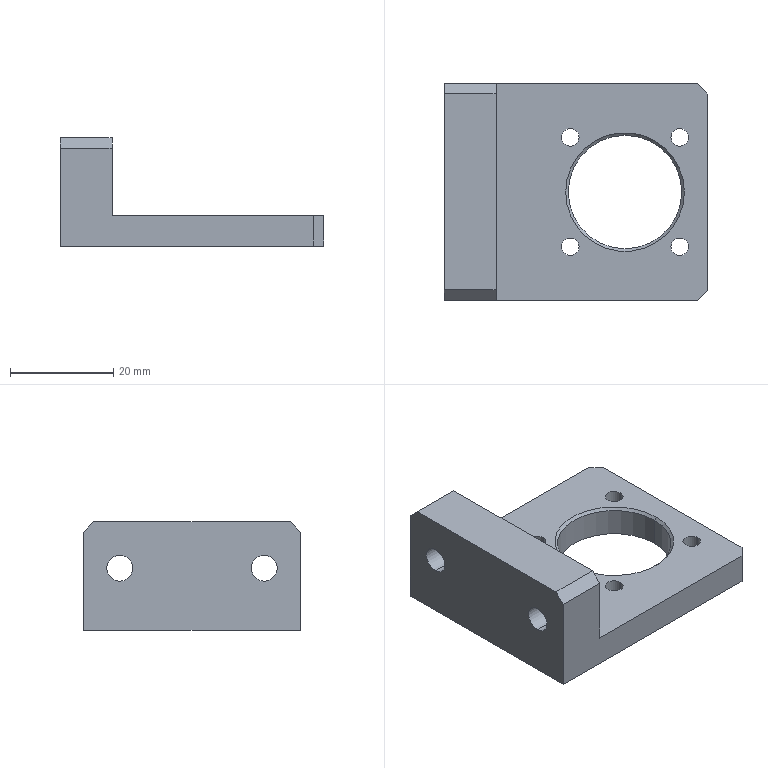Part | NX | features BREP 1 | 1 solid | 40 faces | box 51 x 42 x 21 mm | volume 15776 mm3 | cylinder 22 | plane 16 | cone 2 | commonest cylinder face diameters 3.4 x8 7 x8 5 x4 22 x2
STEP:
#1=CARTESIAN_POINT('',(14.,-21.,6.));
#2=VERTEX_POINT('',#1);
#3=CARTESIAN_POINT('',(16.,-19.,6.));
#4=VERTEX_POINT('',#3);
#5=CARTESIAN_POINT('',(16.,-19.,6.));
#6=DIRECTION('',(0.7071,0.7071,0.));
#7=VECTOR('',#6,1000.);
#8=LINE('',#5,#7);
#9=EDGE_CURVE('',#2,#4,#8,.T.);
#10=ORIENTED_EDGE('',*,*,#9,.F.);
#11=CARTESIAN_POINT('',(14.,-21.,0.));
#12=VERTEX_POINT('',#11);
#13=CARTESIAN_POINT('',(14.,-21.,6.));
#14=DIRECTION('',(0.,0.,1.));
#15=VECTOR('',#14,1000.);
#16=LINE('',#13,#15);
#17=EDGE_CURVE('',#12,#2,#16,.T.);
#18=ORIENTED_EDGE('',*,*,#17,.F.);
#19=CARTESIAN_POINT('',(16.,-19.,0.));
#20=VERTEX_POINT('',#19);
#21=CARTESIAN_POINT('',(17.5,-17.5,0.));
#22=DIRECTION('',(-0.7071,-0.7071,0.));
#23=VECTOR('',#22,1000.);
#24=LINE('',#21,#23);
#25=EDGE_CURVE('',#20,#12,#24,.T.);
#26=ORIENTED_EDGE('',*,*,#25,.F.);
#27=CARTESIAN_POINT('',(16.,-19.,6.));
#28=DIRECTION('',(0.,0.,-1.));
#29=VECTOR('',#28,1000.);
#30=LINE('',#27,#29);
#31=EDGE_CURVE('',#4,#20,#30,.T.);
#32=ORIENTED_EDGE('',*,*,#31,.F.);
#33=EDGE_LOOP('',(#10,#18,#26,#32));
#34=FACE_BOUND('',#33,.T.);
#35=CARTESIAN_POINT('',(16.,-19.,6.));
#36=DIRECTION('',(-0.7071,0.7071,0.));
#37=DIRECTION('',(0.,0.,-1.));
#38=AXIS2_PLACEMENT_3D('',#35,#36,#37);
#39=PLANE('',#38);
#40=ADVANCED_FACE('',(#34),#39,.F.);
#41=CARTESIAN_POINT('',(16.,19.,6.));
#42=VERTEX_POINT('',#41);
#43=CARTESIAN_POINT('',(14.,21.,6.));
#44=VERTEX_POINT('',#43);
#45=CARTESIAN_POINT('',(14.,21.,6.));
#46=DIRECTION('',(-0.7071,0.7071,0.));
#47=VECTOR('',#46,1000.);
#48=LINE('',#45,#47);
#49=EDGE_CURVE('',#42,#44,#48,.T.);
#50=ORIENTED_EDGE('',*,*,#49,.F.);
#51=CARTESIAN_POINT('',(16.,19.,0.));
#52=VERTEX_POINT('',#51);
#53=CARTESIAN_POINT('',(16.,19.,6.));
#54=DIRECTION('',(0.,0.,1.));
#55=VECTOR('',#54,1000.);
#56=LINE('',#53,#55);
#57=EDGE_CURVE('',#52,#42,#56,.T.);
#58=ORIENTED_EDGE('',*,*,#57,.F.);
#59=CARTESIAN_POINT('',(14.,21.,0.));
#60=VERTEX_POINT('',#59);
#61=CARTESIAN_POINT('',(17.5,17.5,0.));
#62=DIRECTION('',(0.7071,-0.7071,0.));
#63=VECTOR('',#62,1000.);
#64=LINE('',#61,#63);
#65=EDGE_CURVE('',#60,#52,#64,.T.);
#66=ORIENTED_EDGE('',*,*,#65,.F.);
#67=CARTESIAN_POINT('',(14.,21.,6.));
#68=DIRECTION('',(0.,0.,-1.));
#69=VECTOR('',#68,1000.);
#70=LINE('',#67,#69);
#71=EDGE_CURVE('',#44,#60,#70,.T.);
#72=ORIENTED_EDGE('',*,*,#71,.F.);
#73=EDGE_LOOP('',(#50,#58,#66,#72));
#74=FACE_BOUND('',#73,.T.);
#75=CARTESIAN_POINT('',(14.,21.,6.));
#76=DIRECTION('',(-0.7071,-0.7071,0.));
#77=DIRECTION('',(0.,0.,-1.));
#78=AXIS2_PLACEMENT_3D('',#75,#76,#77);
#79=PLANE('',#78);
#80=ADVANCED_FACE('',(#74),#79,.F.);
#81=CARTESIAN_POINT('',(-35.,-21.,19.));
#82=VERTEX_POINT('',#81);
#83=CARTESIAN_POINT('',(-35.,-19.,21.));
#84=VERTEX_POINT('',#83);
#85=CARTESIAN_POINT('',(-35.,-19.,21.));
#86=DIRECTION('',(0.,0.7071,0.7071));
#87=VECTOR('',#86,1000.);
#88=LINE('',#85,#87);
#89=EDGE_CURVE('',#82,#84,#88,.T.);
#90=ORIENTED_EDGE('',*,*,#89,.F.);
#91=CARTESIAN_POINT('',(-25.,-21.,19.));
#92=VERTEX_POINT('',#91);
#93=CARTESIAN_POINT('',(-35.,-21.,19.));
#94=DIRECTION('',(-1.,0.,0.));
#95=VECTOR('',#94,1000.);
#96=LINE('',#93,#95);
#97=EDGE_CURVE('',#92,#82,#96,.T.);
#98=ORIENTED_EDGE('',*,*,#97,.F.);
#99=CARTESIAN_POINT('',(-25.,-19.,21.));
#100=VERTEX_POINT('',#99);
#101=CARTESIAN_POINT('',(-25.,-19.,21.));
#102=DIRECTION('',(0.,-0.7071,-0.7071));
#103=VECTOR('',#102,1000.);
#104=LINE('',#101,#103);
#105=EDGE_CURVE('',#100,#92,#104,.T.);
#106=ORIENTED_EDGE('',*,*,#105,.F.);
#107=CARTESIAN_POINT('',(-25.,-19.,21.));
#108=DIRECTION('',(1.,0.,0.));
#109=VECTOR('',#108,1000.);
#110=LINE('',#107,#109);
#111=EDGE_CURVE('',#84,#100,#110,.T.);
#112=ORIENTED_EDGE('',*,*,#111,.F.);
#113=EDGE_LOOP('',(#90,#98,#106,#112));
#114=FACE_BOUND('',#113,.T.);
#115=CARTESIAN_POINT('',(0.,-19.,21.));
#116=DIRECTION('',(0.,-0.7071,0.7071));
#117=DIRECTION('',(-1.,0.,0.));
#118=AXIS2_PLACEMENT_3D('',#115,#116,#117);
#119=PLANE('',#118);
#120=ADVANCED_FACE('',(#114),#119,.T.);
#121=CARTESIAN_POINT('',(-25.,21.,19.));
#122=VERTEX_POINT('',#121);
#123=CARTESIAN_POINT('',(-25.,19.,21.));
#124=VERTEX_POINT('',#123);
#125=CARTESIAN_POINT('',(-25.,19.,21.));
#126=DIRECTION('',(0.,-0.7071,0.7071));
#127=VECTOR('',#126,1000.);
#128=LINE('',#125,#127);
#129=EDGE_CURVE('',#122,#124,#128,.T.);
#130=ORIENTED_EDGE('',*,*,#129,.F.);
#131=CARTESIAN_POINT('',(-35.,21.,19.));
#132=VERTEX_POINT('',#131);
#133=CARTESIAN_POINT('',(-25.,21.,19.));
#134=DIRECTION('',(1.,0.,0.));
#135=VECTOR('',#134,1000.);
#136=LINE('',#133,#135);
#137=EDGE_CURVE('',#132,#122,#136,.T.);
#138=ORIENTED_EDGE('',*,*,#137,.F.);
#139=CARTESIAN_POINT('',(-35.,19.,21.));
#140=VERTEX_POINT('',#139);
#141=CARTESIAN_POINT('',(-35.,19.,21.));
#142=DIRECTION('',(0.,0.7071,-0.7071));
#143=VECTOR('',#142,1000.);
#144=LINE('',#141,#143);
#145=EDGE_CURVE('',#140,#132,#144,.T.);
#146=ORIENTED_EDGE('',*,*,#145,.F.);
#147=CARTESIAN_POINT('',(-35.,19.,21.));
#148=DIRECTION('',(-1.,0.,0.));
#149=VECTOR('',#148,1000.);
#150=LINE('',#147,#149);
#151=EDGE_CURVE('',#124,#140,#150,.T.);
#152=ORIENTED_EDGE('',*,*,#151,.F.);
#153=EDGE_LOOP('',(#130,#138,#146,#152));
#154=FACE_BOUND('',#153,.T.);
#155=CARTESIAN_POINT('',(0.,19.,21.));
#156=DIRECTION('',(0.,0.7071,0.7071));
#157=DIRECTION('',(1.,0.,0.));
#158=AXIS2_PLACEMENT_3D('',#155,#156,#157);
#159=PLANE('',#158);
#160=ADVANCED_FACE('',(#154),#159,.T.);
#161=CARTESIAN_POINT('',(-35.,14.,9.5));
#162=VERTEX_POINT('',#161);
#163=CARTESIAN_POINT('',(-25.,14.,9.5));
#164=VERTEX_POINT('',#163);
#165=CARTESIAN_POINT('',(-35.,14.,9.5));
#166=DIRECTION('',(-1.,0.,0.));
#167=VECTOR('',#166,1000.);
#168=LINE('',#165,#167);
#169=EDGE_CURVE('',#162,#164,#168,.F.);
#170=ORIENTED_EDGE('',*,*,#169,.T.);
#171=CARTESIAN_POINT('',(-25.,14.,14.5));
#172=VERTEX_POINT('',#171);
#173=CARTESIAN_POINT('',(-25.,14.,12.));
#174=DIRECTION('',(-1.,0.,0.));
#175=DIRECTION('',(0.,-1.,0.));
#176=AXIS2_PLACEMENT_3D('',#173,#174,#175);
#177=CIRCLE('',#176,2.5);
#178=EDGE_CURVE('',#172,#164,#177,.T.);
#179=ORIENTED_EDGE('',*,*,#178,.F.);
#180=CARTESIAN_POINT('',(-35.,14.,14.5));
#181=VERTEX_POINT('',#180);
#182=CARTESIAN_POINT('',(-35.,14.,14.5));
#183=DIRECTION('',(-1.,0.,0.));
#184=VECTOR('',#183,1000.);
#185=LINE('',#182,#184);
#186=EDGE_CURVE('',#181,#172,#185,.F.);
#187=ORIENTED_EDGE('',*,*,#186,.F.);
#188=CARTESIAN_POINT('',(-35.,14.,12.));
#189=DIRECTION('',(-1.,0.,0.));
#190=DIRECTION('',(0.,0.,1.));
#191=AXIS2_PLACEMENT_3D('',#188,#189,#190);
#192=CIRCLE('',#191,2.5);
#193=EDGE_CURVE('',#181,#162,#192,.T.);
#194=ORIENTED_EDGE('',*,*,#193,.T.);
#195=EDGE_LOOP('',(#170,#179,#187,#194));
#196=FACE_BOUND('',#195,.T.);
#197=CARTESIAN_POINT('',(-35.,14.,12.));
#198=DIRECTION('',(-1.,0.,0.));
#199=DIRECTION('',(0.,0.,1.));
#200=AXIS2_PLACEMENT_3D('',#197,#198,#199);
#201=CYLINDRICAL_SURFACE('',#200,2.5);
#202=ADVANCED_FACE('',(#196),#201,.F.);
#203=CARTESIAN_POINT('',(-35.,-14.,9.5));
#204=VERTEX_POINT('',#203);
#205=CARTESIAN_POINT('',(-25.,-14.,9.5));
#206=VERTEX_POINT('',#205);
#207=CARTESIAN_POINT('',(-35.,-14.,9.5));
#208=DIRECTION('',(-1.,0.,0.));
#209=VECTOR('',#208,1000.);
#210=LINE('',#207,#209);
#211=EDGE_CURVE('',#204,#206,#210,.F.);
#212=ORIENTED_EDGE('',*,*,#211,.T.);
#213=CARTESIAN_POINT('',(-25.,-14.,14.5));
#214=VERTEX_POINT('',#213);
#215=CARTESIAN_POINT('',(-25.,-14.,12.));
#216=DIRECTION('',(-1.,0.,0.));
#217=DIRECTION('',(0.,-1.,0.));
#218=AXIS2_PLACEMENT_3D('',#215,#216,#217);
#219=CIRCLE('',#218,2.5);
#220=EDGE_CURVE('',#214,#206,#219,.T.);
#221=ORIENTED_EDGE('',*,*,#220,.F.);
#222=CARTESIAN_POINT('',(-35.,-14.,14.5));
#223=VERTEX_POINT('',#222);
#224=CARTESIAN_POINT('',(-35.,-14.,14.5));
#225=DIRECTION('',(-1.,0.,0.));
#226=VECTOR('',#225,1000.);
#227=LINE('',#224,#226);
#228=EDGE_CURVE('',#223,#214,#227,.F.);
#229=ORIENTED_EDGE('',*,*,#228,.F.);
#230=CARTESIAN_POINT('',(-35.,-14.,12.));
#231=DIRECTION('',(-1.,0.,0.));
#232=DIRECTION('',(0.,0.,1.));
#233=AXIS2_PLACEMENT_3D('',#230,#231,#232);
#234=CIRCLE('',#233,2.5);
#235=EDGE_CURVE('',#223,#204,#234,.T.);
#236=ORIENTED_EDGE('',*,*,#235,.T.);
#237=EDGE_LOOP('',(#212,#221,#229,#236));
#238=FACE_BOUND('',#237,.T.);
#239=CARTESIAN_POINT('',(-35.,-14.,12.));
#240=DIRECTION('',(-1.,0.,0.));
#241=DIRECTION('',(0.,0.,1.));
#242=AXIS2_PLACEMENT_3D('',#239,#240,#241);
#243=CYLINDRICAL_SURFACE('',#242,2.5);
#244=ADVANCED_FACE('',(#238),#243,.F.);
#245=CARTESIAN_POINT('',(-11.5,0.,6.));
#246=VERTEX_POINT('',#245);
#247=CARTESIAN_POINT('',(-11.,0.,5.5));
#248=VERTEX_POINT('',#247);
#249=CARTESIAN_POINT('',(-11.,0.,5.5));
#250=DIRECTION('',(-0.7071,0.,0.7071));
#251=VECTOR('',#250,1000.);
#252=LINE('',#249,#251);
#253=EDGE_CURVE('',#246,#248,#252,.F.);
#254=ORIENTED_EDGE('',*,*,#253,.T.);
#255=CARTESIAN_POINT('',(11.,0.,5.5));
#256=VERTEX_POINT('',#255);
#257=CARTESIAN_POINT('',(0.,0.,5.5));
#258=DIRECTION('',(0.,0.,1.));
#259=DIRECTION('',(-1.,0.,0.));
#260=AXIS2_PLACEMENT_3D('',#257,#258,#259);
#261=CIRCLE('',#260,11.);
#262=EDGE_CURVE('',#256,#248,#261,.T.);
#263=ORIENTED_EDGE('',*,*,#262,.F.);
#264=CARTESIAN_POINT('',(11.5,0.,6.));
#265=VERTEX_POINT('',#264);
#266=CARTESIAN_POINT('',(11.,0.,5.5));
#267=DIRECTION('',(0.7071,0.,0.7071));
#268=VECTOR('',#267,1000.);
#269=LINE('',#266,#268);
#270=EDGE_CURVE('',#265,#256,#269,.F.);
#271=ORIENTED_EDGE('',*,*,#270,.F.);
#272=CARTESIAN_POINT('',(0.,0.,6.));
#273=DIRECTION('',(0.,0.,-1.));
#274=DIRECTION('',(-1.,0.,0.));
#275=AXIS2_PLACEMENT_3D('',#272,#273,#274);
#276=CIRCLE('',#275,11.5);
#277=EDGE_CURVE('',#246,#265,#276,.T.);
#278=ORIENTED_EDGE('',*,*,#277,.F.);
#279=EDGE_LOOP('',(#254,#263,#271,#278));
#280=FACE_BOUND('',#279,.T.);
#281=CARTESIAN_POINT('',(0.,0.,5.5));
#282=DIRECTION('',(0.,0.,1.));
#283=DIRECTION('',(1.,0.,0.));
#284=AXIS2_PLACEMENT_3D('',#281,#282,#283);
#285=CONICAL_SURFACE('',#284,11.,0.7854);
#286=ADVANCED_FACE('',(#280),#285,.F.);
#287=CARTESIAN_POINT('',(-7.107,10.607,3.5));
#288=VERTEX_POINT('',#287);
#289=CARTESIAN_POINT('',(-7.107,10.607,0.));
#290=VERTEX_POINT('',#289);
#291=CARTESIAN_POINT('',(-7.107,10.607,0.));
#292=DIRECTION('',(0.,0.,-1.));
#293=VECTOR('',#292,1000.);
#294=LINE('',#291,#293);
#295=EDGE_CURVE('',#288,#290,#294,.T.);
#296=ORIENTED_EDGE('',*,*,#295,.F.);
#297=CARTESIAN_POINT('',(-14.107,10.607,3.5));
#298=VERTEX_POINT('',#297);
#299=CARTESIAN_POINT('',(-10.607,10.607,3.5));
#300=DIRECTION('',(0.,0.,-1.));
#301=DIRECTION('',(-1.,0.,0.));
#302=AXIS2_PLACEMENT_3D('',#299,#300,#301);
#303=CIRCLE('',#302,3.5);
#304=EDGE_CURVE('',#298,#288,#303,.T.);
#305=ORIENTED_EDGE('',*,*,#304,.F.);
#306=CARTESIAN_POINT('',(-14.107,10.607,0.));
#307=VERTEX_POINT('',#306);
#308=CARTESIAN_POINT('',(-14.107,10.607,0.));
#309=DIRECTION('',(0.,0.,-1.));
#310=VECTOR('',#309,1000.);
#311=LINE('',#308,#310);
#312=EDGE_CURVE('',#298,#307,#311,.T.);
#313=ORIENTED_EDGE('',*,*,#312,.T.);
#314=CARTESIAN_POINT('',(-10.607,10.607,0.));
#315=DIRECTION('',(0.,0.,-1.));
#316=DIRECTION('',(-1.,0.,0.));
#317=AXIS2_PLACEMENT_3D('',#314,#315,#316);
#318=CIRCLE('',#317,3.5);
#319=EDGE_CURVE('',#307,#290,#318,.T.);
#320=ORIENTED_EDGE('',*,*,#319,.T.);
#321=EDGE_LOOP('',(#296,#305,#313,#320));
#322=FACE_BOUND('',#321,.T.);
#323=CARTESIAN_POINT('',(-10.607,10.607,0.));
#324=DIRECTION('',(0.,0.,-1.));
#325=DIRECTION('',(-1.,0.,0.));
#326=AXIS2_PLACEMENT_3D('',#323,#324,#325);
#327=CYLINDRICAL_SURFACE('',#326,3.5);
#328=ADVANCED_FACE('',(#322),#327,.F.);
#329=ORIENTED_EDGE('',*,*,#304,.T.);
#330=CARTESIAN_POINT('',(-10.607,10.607,3.5));
#331=DIRECTION('',(0.,0.,-1.));
#332=DIRECTION('',(-1.,0.,0.));
#333=AXIS2_PLACEMENT_3D('',#330,#331,#332);
#334=CIRCLE('',#333,3.5);
#335=EDGE_CURVE('',#288,#298,#334,.T.);
#336=ORIENTED_EDGE('',*,*,#335,.T.);
#337=EDGE_LOOP('',(#329,#336));
#338=FACE_BOUND('',#337,.T.);
#339=CARTESIAN_POINT('',(-12.307,10.607,3.5));
#340=VERTEX_POINT('',#339);
#341=CARTESIAN_POINT('',(-8.907,10.607,3.5));
#342=VERTEX_POINT('',#341);
#343=CARTESIAN_POINT('',(-10.607,10.607,3.5));
#344=DIRECTION('',(0.,0.,-1.));
#345=DIRECTION('',(-1.,0.,0.));
#346=AXIS2_PLACEMENT_3D('',#343,#344,#345);
#347=CIRCLE('',#346,1.7);
#348=EDGE_CURVE('',#340,#342,#347,.T.);
#349=ORIENTED_EDGE('',*,*,#348,.F.);
#350=CARTESIAN_POINT('',(-10.607,10.607,3.5));
#351=DIRECTION('',(0.,0.,-1.));
#352=DIRECTION('',(-1.,0.,0.));
#353=AXIS2_PLACEMENT_3D('',#350,#351,#352);
#354=CIRCLE('',#353,1.7);
#355=EDGE_CURVE('',#342,#340,#354,.T.);
#356=ORIENTED_EDGE('',*,*,#355,.F.);
#357=EDGE_LOOP('',(#349,#356));
#358=FACE_BOUND('',#357,.T.);
#359=CARTESIAN_POINT('',(-8.907,10.607,3.5));
#360=DIRECTION('',(0.,0.,1.));
#361=DIRECTION('',(1.,0.,0.));
#362=AXIS2_PLACEMENT_3D('',#359,#360,#361);
#363=PLANE('',#362);
#364=ADVANCED_FACE('',(#338,#358),#363,.F.);
#365=CARTESIAN_POINT('',(-8.907,10.607,6.));
#366=VERTEX_POINT('',#365);
#367=CARTESIAN_POINT('',(-8.907,10.607,0.));
#368=DIRECTION('',(0.,0.,-1.));
#369=VECTOR('',#368,1000.);
#370=LINE('',#367,#369);
#371=EDGE_CURVE('',#366,#342,#370,.T.);
#372=ORIENTED_EDGE('',*,*,#371,.F.);
#373=CARTESIAN_POINT('',(-12.307,10.607,6.));
#374=VERTEX_POINT('',#373);
#375=CARTESIAN_POINT('',(-10.607,10.607,6.));
#376=DIRECTION('',(0.,0.,-1.));
#377=DIRECTION('',(-1.,0.,0.));
#378=AXIS2_PLACEMENT_3D('',#375,#376,#377);
#379=CIRCLE('',#378,1.7);
#380=EDGE_CURVE('',#374,#366,#379,.T.);
#381=ORIENTED_EDGE('',*,*,#380,.F.);
#382=CARTESIAN_POINT('',(-12.307,10.607,0.));
#383=DIRECTION('',(0.,0.,-1.));
#384=VECTOR('',#383,1000.);
#385=LINE('',#382,#384);
#386=EDGE_CURVE('',#374,#340,#385,.T.);
#387=ORIENTED_EDGE('',*,*,#386,.T.);
#388=ORIENTED_EDGE('',*,*,#348,.T.);
#389=EDGE_LOOP('',(#372,#381,#387,#388));
#390=FACE_BOUND('',#389,.T.);
#391=CARTESIAN_POINT('',(-10.607,10.607,0.));
#392=DIRECTION('',(0.,0.,-1.));
#393=DIRECTION('',(-1.,0.,0.));
#394=AXIS2_PLACEMENT_3D('',#391,#392,#393);
#395=CYLINDRICAL_SURFACE('',#394,1.7);
#396=ADVANCED_FACE('',(#390),#395,.F.);
#397=CARTESIAN_POINT('',(14.107,-10.607,3.5));
#398=VERTEX_POINT('',#397);
#399=CARTESIAN_POINT('',(14.107,-10.607,0.));
#400=VERTEX_POINT('',#399);
#401=CARTESIAN_POINT('',(14.107,-10.607,0.));
#402=DIRECTION('',(0.,0.,-1.));
#403=VECTOR('',#402,1000.);
#404=LINE('',#401,#403);
#405=EDGE_CURVE('',#398,#400,#404,.T.);
#406=ORIENTED_EDGE('',*,*,#405,.F.);
#407=CARTESIAN_POINT('',(7.107,-10.607,3.5));
#408=VERTEX_POINT('',#407);
#409=CARTESIAN_POINT('',(10.607,-10.607,3.5));
#410=DIRECTION('',(0.,0.,-1.));
#411=DIRECTION('',(-1.,0.,0.));
#412=AXIS2_PLACEMENT_3D('',#409,#410,#411);
#413=CIRCLE('',#412,3.5);
#414=EDGE_CURVE('',#408,#398,#413,.T.);
#415=ORIENTED_EDGE('',*,*,#414,.F.);
#416=CARTESIAN_POINT('',(7.107,-10.607,0.));
#417=VERTEX_POINT('',#416);
#418=CARTESIAN_POINT('',(7.107,-10.607,0.));
#419=DIRECTION('',(0.,0.,-1.));
#420=VECTOR('',#419,1000.);
#421=LINE('',#418,#420);
#422=EDGE_CURVE('',#408,#417,#421,.T.);
#423=ORIENTED_EDGE('',*,*,#422,.T.);
#424=CARTESIAN_POINT('',(10.607,-10.607,0.));
#425=DIRECTION('',(0.,0.,-1.));
#426=DIRECTION('',(-1.,0.,0.));
#427=AXIS2_PLACEMENT_3D('',#424,#425,#426);
#428=CIRCLE('',#427,3.5);
#429=EDGE_CURVE('',#417,#400,#428,.T.);
#430=ORIENTED_EDGE('',*,*,#429,.T.);
#431=EDGE_LOOP('',(#406,#415,#423,#430));
#432=FACE_BOUND('',#431,.T.);
#433=CARTESIAN_POINT('',(10.607,-10.607,0.));
#434=DIRECTION('',(0.,0.,-1.));
#435=DIRECTION('',(-1.,0.,0.));
#436=AXIS2_PLACEMENT_3D('',#433,#434,#435);
#437=CYLINDRICAL_SURFACE('',#436,3.5);
#438=ADVANCED_FACE('',(#432),#437,.F.);
#439=ORIENTED_EDGE('',*,*,#414,.T.);
#440=CARTESIAN_POINT('',(10.607,-10.607,3.5));
#441=DIRECTION('',(0.,0.,-1.));
#442=DIRECTION('',(-1.,0.,0.));
#443=AXIS2_PLACEMENT_3D('',#440,#441,#442);
#444=CIRCLE('',#443,3.5);
#445=EDGE_CURVE('',#398,#408,#444,.T.);
#446=ORIENTED_EDGE('',*,*,#445,.T.);
#447=EDGE_LOOP('',(#439,#446));
#448=FACE_BOUND('',#447,.T.);
#449=CARTESIAN_POINT('',(8.907,-10.607,3.5));
#450=VERTEX_POINT('',#449);
#451=CARTESIAN_POINT('',(12.307,-10.607,3.5));
#452=VERTEX_POINT('',#451);
#453=CARTESIAN_POINT('',(10.607,-10.607,3.5));
#454=DIRECTION('',(0.,0.,-1.));
#455=DIRECTION('',(-1.,0.,0.));
#456=AXIS2_PLACEMENT_3D('',#453,#454,#455);
#457=CIRCLE('',#456,1.7);
#458=EDGE_CURVE('',#450,#452,#457,.T.);
#459=ORIENTED_EDGE('',*,*,#458,.F.);
#460=CARTESIAN_POINT('',(10.607,-10.607,3.5));
#461=DIRECTION('',(0.,0.,-1.));
#462=DIRECTION('',(-1.,0.,0.));
#463=AXIS2_PLACEMENT_3D('',#460,#461,#462);
#464=CIRCLE('',#463,1.7);
#465=EDGE_CURVE('',#452,#450,#464,.T.);
#466=ORIENTED_EDGE('',*,*,#465,.F.);
#467=EDGE_LOOP('',(#459,#466));
#468=FACE_BOUND('',#467,.T.);
#469=CARTESIAN_POINT('',(12.307,-10.607,3.5));
#470=DIRECTION('',(0.,0.,1.));
#471=DIRECTION('',(1.,0.,0.));
#472=AXIS2_PLACEMENT_3D('',#469,#470,#471);
#473=PLANE('',#472);
#474=ADVANCED_FACE('',(#448,#468),#473,.F.);
#475=CARTESIAN_POINT('',(12.307,-10.607,6.));
#476=VERTEX_POINT('',#475);
#477=CARTESIAN_POINT('',(12.307,-10.607,0.));
#478=DIRECTION('',(0.,0.,-1.));
#479=VECTOR('',#478,1000.);
#480=LINE('',#477,#479);
#481=EDGE_CURVE('',#476,#452,#480,.T.);
#482=ORIENTED_EDGE('',*,*,#481,.F.);
#483=CARTESIAN_POINT('',(8.907,-10.607,6.));
#484=VERTEX_POINT('',#483);
#485=CARTESIAN_POINT('',(10.607,-10.607,6.));
#486=DIRECTION('',(0.,0.,-1.));
#487=DIRECTION('',(-1.,0.,0.));
#488=AXIS2_PLACEMENT_3D('',#485,#486,#487);
#489=CIRCLE('',#488,1.7);
#490=EDGE_CURVE('',#484,#476,#489,.T.);
#491=ORIENTED_EDGE('',*,*,#490,.F.);
#492=CARTESIAN_POINT('',(8.907,-10.607,0.));
#493=DIRECTION('',(0.,0.,-1.));
#494=VECTOR('',#493,1000.);
#495=LINE('',#492,#494);
#496=EDGE_CURVE('',#484,#450,#495,.T.);
#497=ORIENTED_EDGE('',*,*,#496,.T.);
#498=ORIENTED_EDGE('',*,*,#458,.T.);
#499=EDGE_LOOP('',(#482,#491,#497,#498));
#500=FACE_BOUND('',#499,.T.);
#501=CARTESIAN_POINT('',(10.607,-10.607,0.));
#502=DIRECTION('',(0.,0.,-1.));
#503=DIRECTION('',(-1.,0.,0.));
#504=AXIS2_PLACEMENT_3D('',#501,#502,#503);
#505=CYLINDRICAL_SURFACE('',#504,1.7);
#506=ADVANCED_FACE('',(#500),#505,.F.);
#507=CARTESIAN_POINT('',(14.107,10.607,3.5));
#508=VERTEX_POINT('',#507);
#509=CARTESIAN_POINT('',(14.107,10.607,0.));
#510=VERTEX_POINT('',#509);
#511=CARTESIAN_POINT('',(14.107,10.607,0.));
#512=DIRECTION('',(0.,0.,-1.));
#513=VECTOR('',#512,1000.);
#514=LINE('',#511,#513);
#515=EDGE_CURVE('',#508,#510,#514,.T.);
#516=ORIENTED_EDGE('',*,*,#515,.F.);
#517=CARTESIAN_POINT('',(7.107,10.607,3.5));
#518=VERTEX_POINT('',#517);
#519=CARTESIAN_POINT('',(10.607,10.607,3.5));
#520=DIRECTION('',(0.,0.,-1.));
#521=DIRECTION('',(-1.,0.,0.));
#522=AXIS2_PLACEMENT_3D('',#519,#520,#521);
#523=CIRCLE('',#522,3.5);
#524=EDGE_CURVE('',#518,#508,#523,.T.);
#525=ORIENTED_EDGE('',*,*,#524,.F.);
#526=CARTESIAN_POINT('',(7.107,10.607,0.));
#527=VERTEX_POINT('',#526);
#528=CARTESIAN_POINT('',(7.107,10.607,0.));
#529=DIRECTION('',(0.,0.,-1.));
#530=VECTOR('',#529,1000.);
#531=LINE('',#528,#530);
#532=EDGE_CURVE('',#518,#527,#531,.T.);
#533=ORIENTED_EDGE('',*,*,#532,.T.);
#534=CARTESIAN_POINT('',(10.607,10.607,0.));
#535=DIRECTION('',(0.,0.,-1.));
#536=DIRECTION('',(-1.,0.,0.));
#537=AXIS2_PLACEMENT_3D('',#534,#535,#536);
#538=CIRCLE('',#537,3.5);
#539=EDGE_CURVE('',#527,#510,#538,.T.);
#540=ORIENTED_EDGE('',*,*,#539,.T.);
#541=EDGE_LOOP('',(#516,#525,#533,#540));
#542=FACE_BOUND('',#541,.T.);
#543=CARTESIAN_POINT('',(10.607,10.607,0.));
#544=DIRECTION('',(0.,0.,-1.));
#545=DIRECTION('',(-1.,0.,0.));
#546=AXIS2_PLACEMENT_3D('',#543,#544,#545);
#547=CYLINDRICAL_SURFACE('',#546,3.5);
#548=ADVANCED_FACE('',(#542),#547,.F.);
#549=ORIENTED_EDGE('',*,*,#524,.T.);
#550=CARTESIAN_POINT('',(10.607,10.607,3.5));
#551=DIRECTION('',(0.,0.,-1.));
#552=DIRECTION('',(-1.,0.,0.));
#553=AXIS2_PLACEMENT_3D('',#550,#551,#552);
#554=CIRCLE('',#553,3.5);
#555=EDGE_CURVE('',#508,#518,#554,.T.);
#556=ORIENTED_EDGE('',*,*,#555,.T.);
#557=EDGE_LOOP('',(#549,#556));
#558=FACE_BOUND('',#557,.T.);
#559=CARTESIAN_POINT('',(8.907,10.607,3.5));
#560=VERTEX_POINT('',#559);
#561=CARTESIAN_POINT('',(12.307,10.607,3.5));
#562=VERTEX_POINT('',#561);
#563=CARTESIAN_POINT('',(10.607,10.607,3.5));
#564=DIRECTION('',(0.,0.,-1.));
#565=DIRECTION('',(-1.,0.,0.));
#566=AXIS2_PLACEMENT_3D('',#563,#564,#565);
#567=CIRCLE('',#566,1.7);
#568=EDGE_CURVE('',#560,#562,#567,.T.);
#569=ORIENTED_EDGE('',*,*,#568,.F.);
#570=CARTESIAN_POINT('',(10.607,10.607,3.5));
#571=DIRECTION('',(0.,0.,-1.));
#572=DIRECTION('',(-1.,0.,0.));
#573=AXIS2_PLACEMENT_3D('',#570,#571,#572);
#574=CIRCLE('',#573,1.7);
#575=EDGE_CURVE('',#562,#560,#574,.T.);
#576=ORIENTED_EDGE('',*,*,#575,.F.);
#577=EDGE_LOOP('',(#569,#576));
#578=FACE_BOUND('',#577,.T.);
#579=CARTESIAN_POINT('',(12.307,10.607,3.5));
#580=DIRECTION('',(0.,0.,1.));
#581=DIRECTION('',(1.,0.,0.));
#582=AXIS2_PLACEMENT_3D('',#579,#580,#581);
#583=PLANE('',#582);
#584=ADVANCED_FACE('',(#558,#578),#583,.F.);
#585=CARTESIAN_POINT('',(12.307,10.607,6.));
#586=VERTEX_POINT('',#585);
#587=CARTESIAN_POINT('',(12.307,10.607,0.));
#588=DIRECTION('',(0.,0.,-1.));
#589=VECTOR('',#588,1000.);
#590=LINE('',#587,#589);
#591=EDGE_CURVE('',#586,#562,#590,.T.);
#592=ORIENTED_EDGE('',*,*,#591,.F.);
#593=CARTESIAN_POINT('',(8.907,10.607,6.));
#594=VERTEX_POINT('',#593);
#595=CARTESIAN_POINT('',(10.607,10.607,6.));
#596=DIRECTION('',(0.,0.,-1.));
#597=DIRECTION('',(-1.,0.,0.));
#598=AXIS2_PLACEMENT_3D('',#595,#596,#597);
#599=CIRCLE('',#598,1.7);
#600=EDGE_CURVE('',#594,#586,#599,.T.);
#601=ORIENTED_EDGE('',*,*,#600,.F.);
#602=CARTESIAN_POINT('',(8.907,10.607,0.));
#603=DIRECTION('',(0.,0.,-1.));
#604=VECTOR('',#603,1000.);
#605=LINE('',#602,#604);
#606=EDGE_CURVE('',#594,#560,#605,.T.);
#607=ORIENTED_EDGE('',*,*,#606,.T.);
#608=ORIENTED_EDGE('',*,*,#568,.T.);
#609=EDGE_LOOP('',(#592,#601,#607,#608));
#610=FACE_BOUND('',#609,.T.);
#611=CARTESIAN_POINT('',(10.607,10.607,0.));
#612=DIRECTION('',(0.,0.,-1.));
#613=DIRECTION('',(-1.,0.,0.));
#614=AXIS2_PLACEMENT_3D('',#611,#612,#613);
#615=CYLINDRICAL_SURFACE('',#614,1.7);
#616=ADVANCED_FACE('',(#610),#615,.F.);
#617=CARTESIAN_POINT('',(-7.107,-10.607,3.5));
#618=VERTEX_POINT('',#617);
#619=CARTESIAN_POINT('',(-7.107,-10.607,0.));
#620=VERTEX_POINT('',#619);
#621=CARTESIAN_POINT('',(-7.107,-10.607,0.));
#622=DIRECTION('',(0.,0.,-1.));
#623=VECTOR('',#622,1000.);
#624=LINE('',#621,#623);
#625=EDGE_CURVE('',#618,#620,#624,.T.);
#626=ORIENTED_EDGE('',*,*,#625,.F.);
#627=CARTESIAN_POINT('',(-14.107,-10.607,3.5));
#628=VERTEX_POINT('',#627);
#629=CARTESIAN_POINT('',(-10.607,-10.607,3.5));
#630=DIRECTION('',(0.,0.,-1.));
#631=DIRECTION('',(-1.,0.,0.));
#632=AXIS2_PLACEMENT_3D('',#629,#630,#631);
#633=CIRCLE('',#632,3.5);
#634=EDGE_CURVE('',#628,#618,#633,.T.);
#635=ORIENTED_EDGE('',*,*,#634,.F.);
#636=CARTESIAN_POINT('',(-14.107,-10.607,0.));
#637=VERTEX_POINT('',#636);
#638=CARTESIAN_POINT('',(-14.107,-10.607,0.));
#639=DIRECTION('',(0.,0.,-1.));
#640=VECTOR('',#639,1000.);
#641=LINE('',#638,#640);
#642=EDGE_CURVE('',#628,#637,#641,.T.);
#643=ORIENTED_EDGE('',*,*,#642,.T.);
#644=CARTESIAN_POINT('',(-10.607,-10.607,0.));
#645=DIRECTION('',(0.,0.,-1.));
#646=DIRECTION('',(-1.,0.,0.));
#647=AXIS2_PLACEMENT_3D('',#644,#645,#646);
#648=CIRCLE('',#647,3.5);
#649=EDGE_CURVE('',#637,#620,#648,.T.);
#650=ORIENTED_EDGE('',*,*,#649,.T.);
#651=EDGE_LOOP('',(#626,#635,#643,#650));
#652=FACE_BOUND('',#651,.T.);
#653=CARTESIAN_POINT('',(-10.607,-10.607,0.));
#654=DIRECTION('',(0.,0.,-1.));
#655=DIRECTION('',(-1.,0.,0.));
#656=AXIS2_PLACEMENT_3D('',#653,#654,#655);
#657=CYLINDRICAL_SURFACE('',#656,3.5);
#658=ADVANCED_FACE('',(#652),#657,.F.);
#659=ORIENTED_EDGE('',*,*,#634,.T.);
#660=CARTESIAN_POINT('',(-10.607,-10.607,3.5));
#661=DIRECTION('',(0.,0.,-1.));
#662=DIRECTION('',(-1.,0.,0.));
#663=AXIS2_PLACEMENT_3D('',#660,#661,#662);
#664=CIRCLE('',#663,3.5);
#665=EDGE_CURVE('',#618,#628,#664,.T.);
#666=ORIENTED_EDGE('',*,*,#665,.T.);
#667=EDGE_LOOP('',(#659,#666));
#668=FACE_BOUND('',#667,.T.);
#669=CARTESIAN_POINT('',(-12.307,-10.607,3.5));
#670=VERTEX_POINT('',#669);
#671=CARTESIAN_POINT('',(-8.907,-10.607,3.5));
#672=VERTEX_POINT('',#671);
#673=CARTESIAN_POINT('',(-10.607,-10.607,3.5));
#674=DIRECTION('',(0.,0.,-1.));
#675=DIRECTION('',(-1.,0.,0.));
#676=AXIS2_PLACEMENT_3D('',#673,#674,#675);
#677=CIRCLE('',#676,1.7);
#678=EDGE_CURVE('',#670,#672,#677,.T.);
#679=ORIENTED_EDGE('',*,*,#678,.F.);
#680=CARTESIAN_POINT('',(-10.607,-10.607,3.5));
#681=DIRECTION('',(0.,0.,-1.));
#682=DIRECTION('',(-1.,0.,0.));
#683=AXIS2_PLACEMENT_3D('',#680,#681,#682);
#684=CIRCLE('',#683,1.7);
#685=EDGE_CURVE('',#672,#670,#684,.T.);
#686=ORIENTED_EDGE('',*,*,#685,.F.);
#687=EDGE_LOOP('',(#679,#686));
#688=FACE_BOUND('',#687,.T.);
#689=CARTESIAN_POINT('',(-8.907,-10.607,3.5));
#690=DIRECTION('',(0.,0.,1.));
#691=DIRECTION('',(1.,0.,0.));
#692=AXIS2_PLACEMENT_3D('',#689,#690,#691);
#693=PLANE('',#692);
#694=ADVANCED_FACE('',(#668,#688),#693,.F.);
#695=CARTESIAN_POINT('',(-8.907,-10.607,6.));
#696=VERTEX_POINT('',#695);
#697=CARTESIAN_POINT('',(-8.907,-10.607,0.));
#698=DIRECTION('',(0.,0.,-1.));
#699=VECTOR('',#698,1000.);
#700=LINE('',#697,#699);
#701=EDGE_CURVE('',#696,#672,#700,.T.);
#702=ORIENTED_EDGE('',*,*,#701,.F.);
#703=CARTESIAN_POINT('',(-12.307,-10.607,6.));
#704=VERTEX_POINT('',#703);
#705=CARTESIAN_POINT('',(-10.607,-10.607,6.));
#706=DIRECTION('',(0.,0.,-1.));
#707=DIRECTION('',(-1.,0.,0.));
#708=AXIS2_PLACEMENT_3D('',#705,#706,#707);
#709=CIRCLE('',#708,1.7);
#710=EDGE_CURVE('',#704,#696,#709,.T.);
#711=ORIENTED_EDGE('',*,*,#710,.F.);
#712=CARTESIAN_POINT('',(-12.307,-10.607,0.));
#713=DIRECTION('',(0.,0.,-1.));
#714=VECTOR('',#713,1000.);
#715=LINE('',#712,#714);
#716=EDGE_CURVE('',#704,#670,#715,.T.);
#717=ORIENTED_EDGE('',*,*,#716,.T.);
#718=ORIENTED_EDGE('',*,*,#678,.T.);
#719=EDGE_LOOP('',(#702,#711,#717,#718));
#720=FACE_BOUND('',#719,.T.);
#721=CARTESIAN_POINT('',(-10.607,-10.607,0.));
#722=DIRECTION('',(0.,0.,-1.));
#723=DIRECTION('',(-1.,0.,0.));
#724=AXIS2_PLACEMENT_3D('',#721,#722,#723);
#725=CYLINDRICAL_SURFACE('',#724,1.7);
#726=ADVANCED_FACE('',(#720),#725,.F.);
#727=CARTESIAN_POINT('',(-25.,21.,21.));
#728=DIRECTION('',(0.,1.,0.));
#729=VECTOR('',#728,1000.);
#730=LINE('',#727,#729);
#731=EDGE_CURVE('',#100,#124,#730,.T.);
#732=ORIENTED_EDGE('',*,*,#731,.T.);
#733=ORIENTED_EDGE('',*,*,#151,.T.);
#734=CARTESIAN_POINT('',(-35.,21.,21.));
#735=DIRECTION('',(0.,-1.,0.));
#736=VECTOR('',#735,1000.);
#737=LINE('',#734,#736);
#738=EDGE_CURVE('',#140,#84,#737,.T.);
#739=ORIENTED_EDGE('',*,*,#738,.T.);
#740=ORIENTED_EDGE('',*,*,#111,.T.);
#741=EDGE_LOOP('',(#732,#733,#739,#740));
#742=FACE_BOUND('',#741,.T.);
#743=CARTESIAN_POINT('',(0.,0.,21.));
#744=DIRECTION('',(0.,0.,1.));
#745=DIRECTION('',(1.,0.,0.));
#746=AXIS2_PLACEMENT_3D('',#743,#744,#745);
#747=PLANE('',#746);
#748=ADVANCED_FACE('',(#742),#747,.T.);
#749=CARTESIAN_POINT('',(-25.,21.,6.));
#750=VERTEX_POINT('',#749);
#751=CARTESIAN_POINT('',(-25.,21.,21.));
#752=DIRECTION('',(0.,0.,-1.));
#753=VECTOR('',#752,1000.);
#754=LINE('',#751,#753);
#755=EDGE_CURVE('',#122,#750,#754,.T.);
#756=ORIENTED_EDGE('',*,*,#755,.F.);
#757=ORIENTED_EDGE('',*,*,#129,.T.);
#758=ORIENTED_EDGE('',*,*,#731,.F.);
#759=ORIENTED_EDGE('',*,*,#105,.T.);
#760=CARTESIAN_POINT('',(-25.,-21.,6.));
#761=VERTEX_POINT('',#760);
#762=CARTESIAN_POINT('',(-25.,-21.,21.));
#763=DIRECTION('',(0.,0.,-1.));
#764=VECTOR('',#763,1000.);
#765=LINE('',#762,#764);
#766=EDGE_CURVE('',#92,#761,#765,.T.);
#767=ORIENTED_EDGE('',*,*,#766,.T.);
#768=CARTESIAN_POINT('',(-25.,21.,6.));
#769=DIRECTION('',(0.,1.,0.));
#770=VECTOR('',#769,1000.);
#771=LINE('',#768,#770);
#772=EDGE_CURVE('',#761,#750,#771,.T.);
#773=ORIENTED_EDGE('',*,*,#772,.T.);
#774=EDGE_LOOP('',(#756,#757,#758,#759,#767,#773));
#775=FACE_BOUND('',#774,.T.);
#776=ORIENTED_EDGE('',*,*,#220,.T.);
#777=CARTESIAN_POINT('',(-25.,-14.,12.));
#778=DIRECTION('',(-1.,0.,0.));
#779=DIRECTION('',(0.,-1.,0.));
#780=AXIS2_PLACEMENT_3D('',#777,#778,#779);
#781=CIRCLE('',#780,2.5);
#782=EDGE_CURVE('',#206,#214,#781,.T.);
#783=ORIENTED_EDGE('',*,*,#782,.T.);
#784=EDGE_LOOP('',(#776,#783));
#785=FACE_BOUND('',#784,.T.);
#786=ORIENTED_EDGE('',*,*,#178,.T.);
#787=CARTESIAN_POINT('',(-25.,14.,12.));
#788=DIRECTION('',(-1.,0.,0.));
#789=DIRECTION('',(0.,-1.,0.));
#790=AXIS2_PLACEMENT_3D('',#787,#788,#789);
#791=CIRCLE('',#790,2.5);
#792=EDGE_CURVE('',#164,#172,#791,.T.);
#793=ORIENTED_EDGE('',*,*,#792,.T.);
#794=EDGE_LOOP('',(#786,#793));
#795=FACE_BOUND('',#794,.T.);
#796=CARTESIAN_POINT('',(-25.,21.,21.));
#797=DIRECTION('',(-1.,0.,0.));
#798=DIRECTION('',(0.,-1.,0.));
#799=AXIS2_PLACEMENT_3D('',#796,#797,#798);
#800=PLANE('',#799);
#801=ADVANCED_FACE('',(#775,#785,#795),#800,.F.);
#802=CARTESIAN_POINT('',(11.,0.,0.));
#803=VERTEX_POINT('',#802);
#804=CARTESIAN_POINT('',(11.,0.,6.));
#805=DIRECTION('',(0.,0.,-1.));
#806=VECTOR('',#805,1000.);
#807=LINE('',#804,#806);
#808=EDGE_CURVE('',#256,#803,#807,.T.);
#809=ORIENTED_EDGE('',*,*,#808,.F.);
#810=ORIENTED_EDGE('',*,*,#262,.T.);
#811=CARTESIAN_POINT('',(-11.,0.,0.));
#812=VERTEX_POINT('',#811);
#813=CARTESIAN_POINT('',(-11.,0.,6.));
#814=DIRECTION('',(0.,0.,-1.));
#815=VECTOR('',#814,1000.);
#816=LINE('',#813,#815);
#817=EDGE_CURVE('',#248,#812,#816,.T.);
#818=ORIENTED_EDGE('',*,*,#817,.T.);
#819=CARTESIAN_POINT('',(0.,0.,0.));
#820=DIRECTION('',(0.,0.,1.));
#821=DIRECTION('',(1.,0.,0.));
#822=AXIS2_PLACEMENT_3D('',#819,#820,#821);
#823=CIRCLE('',#822,11.);
#824=EDGE_CURVE('',#803,#812,#823,.T.);
#825=ORIENTED_EDGE('',*,*,#824,.F.);
#826=EDGE_LOOP('',(#809,#810,#818,#825));
#827=FACE_BOUND('',#826,.T.);
#828=CARTESIAN_POINT('',(0.,0.,6.));
#829=DIRECTION('',(0.,0.,-1.));
#830=DIRECTION('',(-1.,0.,0.));
#831=AXIS2_PLACEMENT_3D('',#828,#829,#830);
#832=CYLINDRICAL_SURFACE('',#831,11.);
#833=ADVANCED_FACE('',(#827),#832,.F.);
#834=ORIENTED_EDGE('',*,*,#766,.F.);
#835=ORIENTED_EDGE('',*,*,#97,.T.);
#836=CARTESIAN_POINT('',(-35.,-21.,0.));
#837=VERTEX_POINT('',#836);
#838=CARTESIAN_POINT('',(-35.,-21.,6.));
#839=DIRECTION('',(0.,0.,-1.));
#840=VECTOR('',#839,1000.);
#841=LINE('',#838,#840);
#842=EDGE_CURVE('',#82,#837,#841,.T.);
#843=ORIENTED_EDGE('',*,*,#842,.T.);
#844=CARTESIAN_POINT('',(-35.,-21.,0.));
#845=DIRECTION('',(1.,0.,0.));
#846=VECTOR('',#845,1000.);
#847=LINE('',#844,#846);
#848=EDGE_CURVE('',#837,#12,#847,.T.);
#849=ORIENTED_EDGE('',*,*,#848,.T.);
#850=ORIENTED_EDGE('',*,*,#17,.T.);
#851=CARTESIAN_POINT('',(-35.,-21.,6.));
#852=DIRECTION('',(1.,0.,0.));
#853=VECTOR('',#852,1000.);
#854=LINE('',#851,#853);
#855=EDGE_CURVE('',#761,#2,#854,.T.);
#856=ORIENTED_EDGE('',*,*,#855,.F.);
#857=EDGE_LOOP('',(#834,#835,#843,#849,#850,#856));
#858=FACE_BOUND('',#857,.T.);
#859=CARTESIAN_POINT('',(-35.,-21.,6.));
#860=DIRECTION('',(0.,1.,0.));
#861=DIRECTION('',(-1.,0.,0.));
#862=AXIS2_PLACEMENT_3D('',#859,#860,#861);
#863=PLANE('',#862);
#864=ADVANCED_FACE('',(#858),#863,.F.);
#865=ORIENTED_EDGE('',*,*,#738,.F.);
#866=ORIENTED_EDGE('',*,*,#145,.T.);
#867=CARTESIAN_POINT('',(-35.,21.,0.));
#868=VERTEX_POINT('',#867);
#869=CARTESIAN_POINT('',(-35.,21.,6.));
#870=DIRECTION('',(0.,0.,-1.));
#871=VECTOR('',#870,1000.);
#872=LINE('',#869,#871);
#873=EDGE_CURVE('',#132,#868,#872,.T.);
#874=ORIENTED_EDGE('',*,*,#873,.T.);
#875=CARTESIAN_POINT('',(-35.,-21.,0.));
#876=DIRECTION('',(0.,-1.,0.));
#877=VECTOR('',#876,1000.);
#878=LINE('',#875,#877);
#879=EDGE_CURVE('',#868,#837,#878,.T.);
#880=ORIENTED_EDGE('',*,*,#879,.T.);
#881=ORIENTED_EDGE('',*,*,#842,.F.);
#882=ORIENTED_EDGE('',*,*,#89,.T.);
#883=EDGE_LOOP('',(#865,#866,#874,#880,#881,#882));
#884=FACE_BOUND('',#883,.T.);
#885=ORIENTED_EDGE('',*,*,#235,.F.);
#886=CARTESIAN_POINT('',(-35.,-14.,12.));
#887=DIRECTION('',(-1.,0.,0.));
#888=DIRECTION('',(0.,0.,1.));
#889=AXIS2_PLACEMENT_3D('',#886,#887,#888);
#890=CIRCLE('',#889,2.5);
#891=EDGE_CURVE('',#204,#223,#890,.T.);
#892=ORIENTED_EDGE('',*,*,#891,.F.);
#893=EDGE_LOOP('',(#885,#892));
#894=FACE_BOUND('',#893,.T.);
#895=ORIENTED_EDGE('',*,*,#193,.F.);
#896=CARTESIAN_POINT('',(-35.,14.,12.));
#897=DIRECTION('',(-1.,0.,0.));
#898=DIRECTION('',(0.,0.,1.));
#899=AXIS2_PLACEMENT_3D('',#896,#897,#898);
#900=CIRCLE('',#899,2.5);
#901=EDGE_CURVE('',#162,#181,#900,.T.);
#902=ORIENTED_EDGE('',*,*,#901,.F.);
#903=EDGE_LOOP('',(#895,#902));
#904=FACE_BOUND('',#903,.T.);
#905=CARTESIAN_POINT('',(-35.,-21.,6.));
#906=DIRECTION('',(1.,0.,0.));
#907=DIRECTION('',(0.,0.,-1.));
#908=AXIS2_PLACEMENT_3D('',#905,#906,#907);
#909=PLANE('',#908);
#910=ADVANCED_FACE('',(#884,#894,#904),#909,.F.);
#911=ORIENTED_EDGE('',*,*,#873,.F.);
#912=ORIENTED_EDGE('',*,*,#137,.T.);
#913=ORIENTED_EDGE('',*,*,#755,.T.);
#914=CARTESIAN_POINT('',(-35.,21.,6.));
#915=DIRECTION('',(-1.,0.,0.));
#916=VECTOR('',#915,1000.);
#917=LINE('',#914,#916);
#918=EDGE_CURVE('',#44,#750,#917,.T.);
#919=ORIENTED_EDGE('',*,*,#918,.F.);
#920=ORIENTED_EDGE('',*,*,#71,.T.);
#921=CARTESIAN_POINT('',(-35.,21.,0.));
#922=DIRECTION('',(-1.,0.,0.));
#923=VECTOR('',#922,1000.);
#924=LINE('',#921,#923);
#925=EDGE_CURVE('',#60,#868,#924,.T.);
#926=ORIENTED_EDGE('',*,*,#925,.T.);
#927=EDGE_LOOP('',(#911,#912,#913,#919,#920,#926));
#928=FACE_BOUND('',#927,.T.);
#929=CARTESIAN_POINT('',(-35.,21.,6.));
#930=DIRECTION('',(0.,-1.,0.));
#931=DIRECTION('',(1.,0.,0.));
#932=AXIS2_PLACEMENT_3D('',#929,#930,#931);
#933=PLANE('',#932);
#934=ADVANCED_FACE('',(#928),#933,.F.);
#935=CARTESIAN_POINT('',(16.,-21.,0.));
#936=DIRECTION('',(0.,1.,0.));
#937=VECTOR('',#936,1000.);
#938=LINE('',#935,#937);
#939=EDGE_CURVE('',#20,#52,#938,.T.);
#940=ORIENTED_EDGE('',*,*,#939,.T.);
#941=ORIENTED_EDGE('',*,*,#57,.T.);
#942=CARTESIAN_POINT('',(16.,-21.,6.));
#943=DIRECTION('',(0.,1.,0.));
#944=VECTOR('',#943,1000.);
#945=LINE('',#942,#944);
#946=EDGE_CURVE('',#4,#42,#945,.T.);
#947=ORIENTED_EDGE('',*,*,#946,.F.);
#948=ORIENTED_EDGE('',*,*,#31,.T.);
#949=EDGE_LOOP('',(#940,#941,#947,#948));
#950=FACE_BOUND('',#949,.T.);
#951=CARTESIAN_POINT('',(16.,-21.,6.));
#952=DIRECTION('',(-1.,0.,0.));
#953=DIRECTION('',(0.,-1.,0.));
#954=AXIS2_PLACEMENT_3D('',#951,#952,#953);
#955=PLANE('',#954);
#956=ADVANCED_FACE('',(#950),#955,.F.);
#957=CARTESIAN_POINT('',(0.,0.,0.));
#958=DIRECTION('',(0.,0.,1.));
#959=DIRECTION('',(1.,0.,0.));
#960=AXIS2_PLACEMENT_3D('',#957,#958,#959);
#961=CIRCLE('',#960,11.);
#962=EDGE_CURVE('',#812,#803,#961,.T.);
#963=ORIENTED_EDGE('',*,*,#962,.T.);
#964=ORIENTED_EDGE('',*,*,#824,.T.);
#965=EDGE_LOOP('',(#963,#964));
#966=FACE_BOUND('',#965,.T.);
#967=ORIENTED_EDGE('',*,*,#925,.F.);
#968=ORIENTED_EDGE('',*,*,#65,.T.);
#969=ORIENTED_EDGE('',*,*,#939,.F.);
#970=ORIENTED_EDGE('',*,*,#25,.T.);
#971=ORIENTED_EDGE('',*,*,#848,.F.);
#972=ORIENTED_EDGE('',*,*,#879,.F.);
#973=EDGE_LOOP('',(#967,#968,#969,#970,#971,#972));
#974=FACE_BOUND('',#973,.T.);
#975=ORIENTED_EDGE('',*,*,#649,.F.);
#976=CARTESIAN_POINT('',(-10.607,-10.607,0.));
#977=DIRECTION('',(0.,0.,-1.));
#978=DIRECTION('',(-1.,0.,0.));
#979=AXIS2_PLACEMENT_3D('',#976,#977,#978);
#980=CIRCLE('',#979,3.5);
#981=EDGE_CURVE('',#620,#637,#980,.T.);
#982=ORIENTED_EDGE('',*,*,#981,.F.);
#983=EDGE_LOOP('',(#975,#982));
#984=FACE_BOUND('',#983,.T.);
#985=ORIENTED_EDGE('',*,*,#539,.F.);
#986=CARTESIAN_POINT('',(10.607,10.607,0.));
#987=DIRECTION('',(0.,0.,-1.));
#988=DIRECTION('',(-1.,0.,0.));
#989=AXIS2_PLACEMENT_3D('',#986,#987,#988);
#990=CIRCLE('',#989,3.5);
#991=EDGE_CURVE('',#510,#527,#990,.T.);
#992=ORIENTED_EDGE('',*,*,#991,.F.);
#993=EDGE_LOOP('',(#985,#992));
#994=FACE_BOUND('',#993,.T.);
#995=ORIENTED_EDGE('',*,*,#429,.F.);
#996=CARTESIAN_POINT('',(10.607,-10.607,0.));
#997=DIRECTION('',(0.,0.,-1.));
#998=DIRECTION('',(-1.,0.,0.));
#999=AXIS2_PLACEMENT_3D('',#996,#997,#998);
#1000=CIRCLE('',#999,3.5);
#1001=EDGE_CURVE('',#400,#417,#1000,.T.);
#1002=ORIENTED_EDGE('',*,*,#1001,.F.);
#1003=EDGE_LOOP('',(#995,#1002));
#1004=FACE_BOUND('',#1003,.T.);
#1005=ORIENTED_EDGE('',*,*,#319,.F.);
#1006=CARTESIAN_POINT('',(-10.607,10.607,0.));
#1007=DIRECTION('',(0.,0.,-1.));
#1008=DIRECTION('',(-1.,0.,0.));
#1009=AXIS2_PLACEMENT_3D('',#1006,#1007,#1008);
#1010=CIRCLE('',#1009,3.5);
#1011=EDGE_CURVE('',#290,#307,#1010,.T.);
#1012=ORIENTED_EDGE('',*,*,#1011,.F.);
#1013=EDGE_LOOP('',(#1005,#1012));
#1014=FACE_BOUND('',#1013,.T.);
#1015=CARTESIAN_POINT('',(0.,0.,0.));
#1016=DIRECTION('',(0.,0.,-1.));
#1017=DIRECTION('',(-1.,0.,0.));
#1018=AXIS2_PLACEMENT_3D('',#1015,#1016,#1017);
#1019=PLANE('',#1018);
#1020=ADVANCED_FACE('',(#966,#974,#984,#994,#1004,#1014),#1019,.T.);
#1021=ORIENTED_EDGE('',*,*,#946,.T.);
#1022=ORIENTED_EDGE('',*,*,#49,.T.);
#1023=ORIENTED_EDGE('',*,*,#918,.T.);
#1024=ORIENTED_EDGE('',*,*,#772,.F.);
#1025=ORIENTED_EDGE('',*,*,#855,.T.);
#1026=ORIENTED_EDGE('',*,*,#9,.T.);
#1027=EDGE_LOOP('',(#1021,#1022,#1023,#1024,#1025,#1026));
#1028=FACE_BOUND('',#1027,.T.);
#1029=ORIENTED_EDGE('',*,*,#710,.T.);
#1030=CARTESIAN_POINT('',(-10.607,-10.607,6.));
#1031=DIRECTION('',(0.,0.,-1.));
#1032=DIRECTION('',(-1.,0.,0.));
#1033=AXIS2_PLACEMENT_3D('',#1030,#1031,#1032);
#1034=CIRCLE('',#1033,1.7);
#1035=EDGE_CURVE('',#696,#704,#1034,.T.);
#1036=ORIENTED_EDGE('',*,*,#1035,.T.);
#1037=EDGE_LOOP('',(#1029,#1036));
#1038=FACE_BOUND('',#1037,.T.);
#1039=ORIENTED_EDGE('',*,*,#600,.T.);
#1040=CARTESIAN_POINT('',(10.607,10.607,6.));
#1041=DIRECTION('',(0.,0.,-1.));
#1042=DIRECTION('',(-1.,0.,0.));
#1043=AXIS2_PLACEMENT_3D('',#1040,#1041,#1042);
#1044=CIRCLE('',#1043,1.7);
#1045=EDGE_CURVE('',#586,#594,#1044,.T.);
#1046=ORIENTED_EDGE('',*,*,#1045,.T.);
#1047=EDGE_LOOP('',(#1039,#1046));
#1048=FACE_BOUND('',#1047,.T.);
#1049=ORIENTED_EDGE('',*,*,#490,.T.);
#1050=CARTESIAN_POINT('',(10.607,-10.607,6.));
#1051=DIRECTION('',(0.,0.,-1.));
#1052=DIRECTION('',(-1.,0.,0.));
#1053=AXIS2_PLACEMENT_3D('',#1050,#1051,#1052);
#1054=CIRCLE('',#1053,1.7);
#1055=EDGE_CURVE('',#476,#484,#1054,.T.);
#1056=ORIENTED_EDGE('',*,*,#1055,.T.);
#1057=EDGE_LOOP('',(#1049,#1056));
#1058=FACE_BOUND('',#1057,.T.);
#1059=ORIENTED_EDGE('',*,*,#380,.T.);
#1060=CARTESIAN_POINT('',(-10.607,10.607,6.));
#1061=DIRECTION('',(0.,0.,-1.));
#1062=DIRECTION('',(-1.,0.,0.));
#1063=AXIS2_PLACEMENT_3D('',#1060,#1061,#1062);
#1064=CIRCLE('',#1063,1.7);
#1065=EDGE_CURVE('',#366,#374,#1064,.T.);
#1066=ORIENTED_EDGE('',*,*,#1065,.T.);
#1067=EDGE_LOOP('',(#1059,#1066));
#1068=FACE_BOUND('',#1067,.T.);
#1069=CARTESIAN_POINT('',(0.,0.,6.));
#1070=DIRECTION('',(0.,0.,-1.));
#1071=DIRECTION('',(-1.,0.,0.));
#1072=AXIS2_PLACEMENT_3D('',#1069,#1070,#1071);
#1073=CIRCLE('',#1072,11.5);
#1074=EDGE_CURVE('',#265,#246,#1073,.T.);
#1075=ORIENTED_EDGE('',*,*,#1074,.T.);
#1076=ORIENTED_EDGE('',*,*,#277,.T.);
#1077=EDGE_LOOP('',(#1075,#1076));
#1078=FACE_BOUND('',#1077,.T.);
#1079=CARTESIAN_POINT('',(0.,0.,6.));
#1080=DIRECTION('',(0.,0.,-1.));
#1081=DIRECTION('',(-1.,0.,0.));
#1082=AXIS2_PLACEMENT_3D('',#1079,#1080,#1081);
#1083=PLANE('',#1082);
#1084=ADVANCED_FACE('',(#1028,#1038,#1048,#1058,#1068,#1078),#1083,.F.);
#1085=CARTESIAN_POINT('',(0.,0.,5.5));
#1086=DIRECTION('',(0.,0.,1.));
#1087=DIRECTION('',(-1.,0.,0.));
#1088=AXIS2_PLACEMENT_3D('',#1085,#1086,#1087);
#1089=CIRCLE('',#1088,11.);
#1090=EDGE_CURVE('',#248,#256,#1089,.T.);
#1091=ORIENTED_EDGE('',*,*,#1090,.T.);
#1092=ORIENTED_EDGE('',*,*,#808,.T.);
#1093=ORIENTED_EDGE('',*,*,#962,.F.);
#1094=ORIENTED_EDGE('',*,*,#817,.F.);
#1095=EDGE_LOOP('',(#1091,#1092,#1093,#1094));
#1096=FACE_BOUND('',#1095,.T.);
#1097=CARTESIAN_POINT('',(0.,0.,6.));
#1098=DIRECTION('',(0.,0.,-1.));
#1099=DIRECTION('',(-1.,0.,0.));
#1100=AXIS2_PLACEMENT_3D('',#1097,#1098,#1099);
#1101=CYLINDRICAL_SURFACE('',#1100,11.);
#1102=ADVANCED_FACE('',(#1096),#1101,.F.);
#1103=ORIENTED_EDGE('',*,*,#1035,.F.);
#1104=ORIENTED_EDGE('',*,*,#701,.T.);
#1105=ORIENTED_EDGE('',*,*,#685,.T.);
#1106=ORIENTED_EDGE('',*,*,#716,.F.);
#1107=EDGE_LOOP('',(#1103,#1104,#1105,#1106));
#1108=FACE_BOUND('',#1107,.T.);
#1109=CARTESIAN_POINT('',(-10.607,-10.607,0.));
#1110=DIRECTION('',(0.,0.,-1.));
#1111=DIRECTION('',(-1.,0.,0.));
#1112=AXIS2_PLACEMENT_3D('',#1109,#1110,#1111);
#1113=CYLINDRICAL_SURFACE('',#1112,1.7);
#1114=ADVANCED_FACE('',(#1108),#1113,.F.);
#1115=ORIENTED_EDGE('',*,*,#665,.F.);
#1116=ORIENTED_EDGE('',*,*,#625,.T.);
#1117=ORIENTED_EDGE('',*,*,#981,.T.);
#1118=ORIENTED_EDGE('',*,*,#642,.F.);
#1119=EDGE_LOOP('',(#1115,#1116,#1117,#1118));
#1120=FACE_BOUND('',#1119,.T.);
#1121=CARTESIAN_POINT('',(-10.607,-10.607,0.));
#1122=DIRECTION('',(0.,0.,-1.));
#1123=DIRECTION('',(-1.,0.,0.));
#1124=AXIS2_PLACEMENT_3D('',#1121,#1122,#1123);
#1125=CYLINDRICAL_SURFACE('',#1124,3.5);
#1126=ADVANCED_FACE('',(#1120),#1125,.F.);
#1127=ORIENTED_EDGE('',*,*,#1045,.F.);
#1128=ORIENTED_EDGE('',*,*,#591,.T.);
#1129=ORIENTED_EDGE('',*,*,#575,.T.);
#1130=ORIENTED_EDGE('',*,*,#606,.F.);
#1131=EDGE_LOOP('',(#1127,#1128,#1129,#1130));
#1132=FACE_BOUND('',#1131,.T.);
#1133=CARTESIAN_POINT('',(10.607,10.607,0.));
#1134=DIRECTION('',(0.,0.,-1.));
#1135=DIRECTION('',(-1.,0.,0.));
#1136=AXIS2_PLACEMENT_3D('',#1133,#1134,#1135);
#1137=CYLINDRICAL_SURFACE('',#1136,1.7);
#1138=ADVANCED_FACE('',(#1132),#1137,.F.);
#1139=ORIENTED_EDGE('',*,*,#555,.F.);
#1140=ORIENTED_EDGE('',*,*,#515,.T.);
#1141=ORIENTED_EDGE('',*,*,#991,.T.);
#1142=ORIENTED_EDGE('',*,*,#532,.F.);
#1143=EDGE_LOOP('',(#1139,#1140,#1141,#1142));
#1144=FACE_BOUND('',#1143,.T.);
#1145=CARTESIAN_POINT('',(10.607,10.607,0.));
#1146=DIRECTION('',(0.,0.,-1.));
#1147=DIRECTION('',(-1.,0.,0.));
#1148=AXIS2_PLACEMENT_3D('',#1145,#1146,#1147);
#1149=CYLINDRICAL_SURFACE('',#1148,3.5);
#1150=ADVANCED_FACE('',(#1144),#1149,.F.);
#1151=ORIENTED_EDGE('',*,*,#1055,.F.);
#1152=ORIENTED_EDGE('',*,*,#481,.T.);
#1153=ORIENTED_EDGE('',*,*,#465,.T.);
#1154=ORIENTED_EDGE('',*,*,#496,.F.);
#1155=EDGE_LOOP('',(#1151,#1152,#1153,#1154));
#1156=FACE_BOUND('',#1155,.T.);
#1157=CARTESIAN_POINT('',(10.607,-10.607,0.));
#1158=DIRECTION('',(0.,0.,-1.));
#1159=DIRECTION('',(-1.,0.,0.));
#1160=AXIS2_PLACEMENT_3D('',#1157,#1158,#1159);
#1161=CYLINDRICAL_SURFACE('',#1160,1.7);
#1162=ADVANCED_FACE('',(#1156),#1161,.F.);
#1163=ORIENTED_EDGE('',*,*,#445,.F.);
#1164=ORIENTED_EDGE('',*,*,#405,.T.);
#1165=ORIENTED_EDGE('',*,*,#1001,.T.);
#1166=ORIENTED_EDGE('',*,*,#422,.F.);
#1167=EDGE_LOOP('',(#1163,#1164,#1165,#1166));
#1168=FACE_BOUND('',#1167,.T.);
#1169=CARTESIAN_POINT('',(10.607,-10.607,0.));
#1170=DIRECTION('',(0.,0.,-1.));
#1171=DIRECTION('',(-1.,0.,0.));
#1172=AXIS2_PLACEMENT_3D('',#1169,#1170,#1171);
#1173=CYLINDRICAL_SURFACE('',#1172,3.5);
#1174=ADVANCED_FACE('',(#1168),#1173,.F.);
#1175=ORIENTED_EDGE('',*,*,#1065,.F.);
#1176=ORIENTED_EDGE('',*,*,#371,.T.);
#1177=ORIENTED_EDGE('',*,*,#355,.T.);
#1178=ORIENTED_EDGE('',*,*,#386,.F.);
#1179=EDGE_LOOP('',(#1175,#1176,#1177,#1178));
#1180=FACE_BOUND('',#1179,.T.);
#1181=CARTESIAN_POINT('',(-10.607,10.607,0.));
#1182=DIRECTION('',(0.,0.,-1.));
#1183=DIRECTION('',(-1.,0.,0.));
#1184=AXIS2_PLACEMENT_3D('',#1181,#1182,#1183);
#1185=CYLINDRICAL_SURFACE('',#1184,1.7);
#1186=ADVANCED_FACE('',(#1180),#1185,.F.);
#1187=ORIENTED_EDGE('',*,*,#335,.F.);
#1188=ORIENTED_EDGE('',*,*,#295,.T.);
#1189=ORIENTED_EDGE('',*,*,#1011,.T.);
#1190=ORIENTED_EDGE('',*,*,#312,.F.);
#1191=EDGE_LOOP('',(#1187,#1188,#1189,#1190));
#1192=FACE_BOUND('',#1191,.T.);
#1193=CARTESIAN_POINT('',(-10.607,10.607,0.));
#1194=DIRECTION('',(0.,0.,-1.));
#1195=DIRECTION('',(-1.,0.,0.));
#1196=AXIS2_PLACEMENT_3D('',#1193,#1194,#1195);
#1197=CYLINDRICAL_SURFACE('',#1196,3.5);
#1198=ADVANCED_FACE('',(#1192),#1197,.F.);
#1199=ORIENTED_EDGE('',*,*,#1090,.F.);
#1200=ORIENTED_EDGE('',*,*,#253,.F.);
#1201=ORIENTED_EDGE('',*,*,#1074,.F.);
#1202=ORIENTED_EDGE('',*,*,#270,.T.);
#1203=EDGE_LOOP('',(#1199,#1200,#1201,#1202));
#1204=FACE_BOUND('',#1203,.T.);
#1205=CARTESIAN_POINT('',(0.,0.,5.5));
#1206=DIRECTION('',(0.,0.,1.));
#1207=DIRECTION('',(1.,0.,0.));
#1208=AXIS2_PLACEMENT_3D('',#1205,#1206,#1207);
#1209=CONICAL_SURFACE('',#1208,11.,0.7854);
#1210=ADVANCED_FACE('',(#1204),#1209,.F.);
#1211=ORIENTED_EDGE('',*,*,#782,.F.);
#1212=ORIENTED_EDGE('',*,*,#211,.F.);
#1213=ORIENTED_EDGE('',*,*,#891,.T.);
#1214=ORIENTED_EDGE('',*,*,#228,.T.);
#1215=EDGE_LOOP('',(#1211,#1212,#1213,#1214));
#1216=FACE_BOUND('',#1215,.T.);
#1217=CARTESIAN_POINT('',(-35.,-14.,12.));
#1218=DIRECTION('',(-1.,0.,0.));
#1219=DIRECTION('',(0.,0.,1.));
#1220=AXIS2_PLACEMENT_3D('',#1217,#1218,#1219);
#1221=CYLINDRICAL_SURFACE('',#1220,2.5);
#1222=ADVANCED_FACE('',(#1216),#1221,.F.);
#1223=ORIENTED_EDGE('',*,*,#792,.F.);
#1224=ORIENTED_EDGE('',*,*,#169,.F.);
#1225=ORIENTED_EDGE('',*,*,#901,.T.);
#1226=ORIENTED_EDGE('',*,*,#186,.T.);
#1227=EDGE_LOOP('',(#1223,#1224,#1225,#1226));
#1228=FACE_BOUND('',#1227,.T.);
#1229=CARTESIAN_POINT('',(-35.,14.,12.));
#1230=DIRECTION('',(-1.,0.,0.));
#1231=DIRECTION('',(0.,0.,1.));
#1232=AXIS2_PLACEMENT_3D('',#1229,#1230,#1231);
#1233=CYLINDRICAL_SURFACE('',#1232,2.5);
#1234=ADVANCED_FACE('',(#1228),#1233,.F.);
#1235=CLOSED_SHELL('',(#40,#80,#120,#160,#202,#244,#286,#328,#364,#396,#438,#474,#506,#548,#584,#616,#658,#694,#726,#748,#801,#833,#864,#910,#934,#956,#1020,#1084,#1102,#1114,#1126,#1138,#1150,#1162,#1174,#1186,#1198,#1210,#1222,#1234));
#1236=MANIFOLD_SOLID_BREP('',#1235);
#1237=(LENGTH_UNIT()NAMED_UNIT(*)SI_UNIT(.MILLI.,.METRE.));
#1238=UNCERTAINTY_MEASURE_WITH_UNIT(LENGTH_MEASURE(0.00001),#1237,'','');
#1239=(NAMED_UNIT(*)PLANE_ANGLE_UNIT()SI_UNIT($,.RADIAN.));
#1240=(NAMED_UNIT(*)SI_UNIT($,.STERADIAN.)SOLID_ANGLE_UNIT());
#1241=(GEOMETRIC_REPRESENTATION_CONTEXT(3)GLOBAL_UNCERTAINTY_ASSIGNED_CONTEXT((#1238))GLOBAL_UNIT_ASSIGNED_CONTEXT((#1237,#1239,#1240))REPRESENTATION_CONTEXT('',''));
#1242=ADVANCED_BREP_SHAPE_REPRESENTATION('',(#1236),#1241);